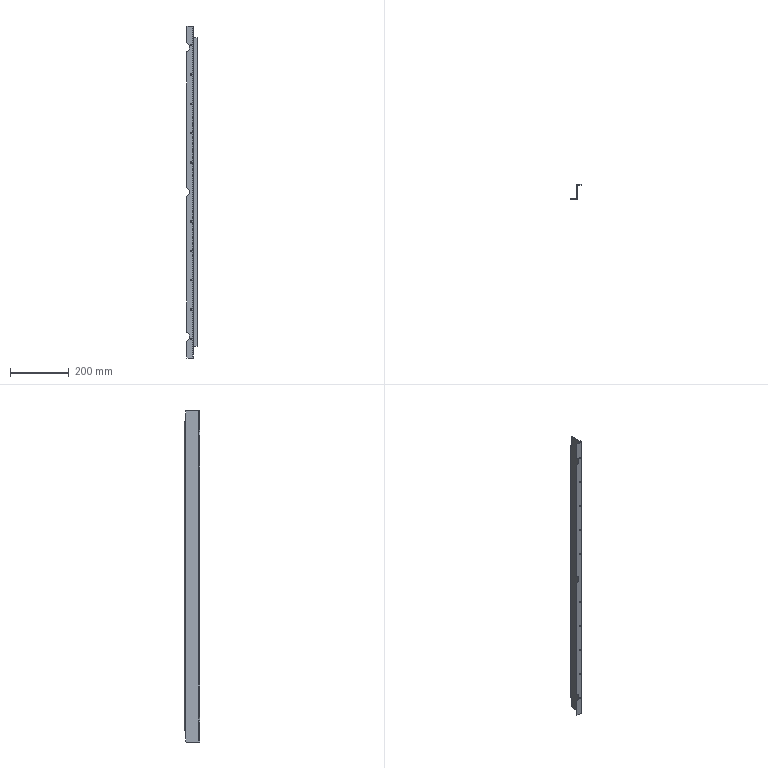Part | SolidWorks | features ICE 4, Chamfer 1, FlatPattern 1, SMBaseFlange 1, SheetMetal 1 | 1 solid | 50 faces | box 35 x 51.5 x 1130 mm | volume 184167 mm3 | cylinder 27 | plane 23 | commonest cylinder face diameters 5 x20 35 x3 0.4 x2 4.4 x2